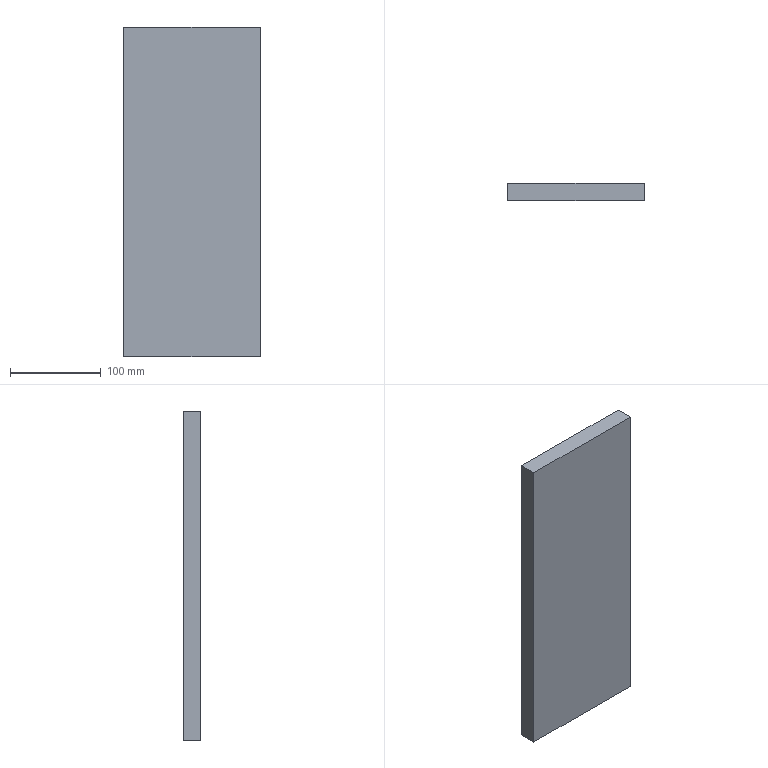Part | STEP file | SN10_010_005-02_PLACA | 1 solid | 6 faces | box 150 x 19 x 362.5 mm | volume 1033125 mm3 | plane 6
STEP:
#1=CARTESIAN_POINT('',(0.,0.,0.));
#2=DIRECTION('',(0.,0.,1.));
#3=DIRECTION('',(1.,0.,0.));
#4=AXIS2_PLACEMENT_3D('',#1,#2,#3);
#5=CARTESIAN_POINT('',(-75.,-419.,379.5));
#6=VERTEX_POINT('',#5);
#7=CARTESIAN_POINT('',(75.,-419.,379.5));
#8=VERTEX_POINT('',#7);
#9=CARTESIAN_POINT('',(-75.,-419.,379.5));
#10=DIRECTION('',(1.,0.,0.));
#11=VECTOR('',#10,1.);
#12=LINE('',#9,#11);
#13=CARTESIAN_POINT('',(0.,-419.,379.5));
#14=DIRECTION('',(0.,-1.,0.));
#15=DIRECTION('',(0.,0.,-1.));
#16=AXIS2_PLACEMENT_3D('',#13,#14,#15);
#17=PLANE('',#16);
#18=CARTESIAN_POINT('',(0.,-75.));
#19=DIRECTION('',(0.,1.));
#20=VECTOR('',#19,1.);
#21=LINE('',#18,#20);
#22=(GEOMETRIC_REPRESENTATION_CONTEXT(2)PARAMETRIC_REPRESENTATION_CONTEXT()REPRESENTATION_CONTEXT('',''));
#23=DEFINITIONAL_REPRESENTATION('',(#21),#22);
#24=PCURVE('',#17,#23);
#25=CARTESIAN_POINT('',(0.,-419.,379.5));
#26=DIRECTION('',(0.,0.,-1.));
#27=DIRECTION('',(-1.,0.,0.));
#28=AXIS2_PLACEMENT_3D('',#25,#26,#27);
#29=PLANE('',#28);
#30=CARTESIAN_POINT('',(75.,0.));
#31=DIRECTION('',(-1.,0.));
#32=VECTOR('',#31,1.);
#33=LINE('',#30,#32);
#34=(GEOMETRIC_REPRESENTATION_CONTEXT(2)PARAMETRIC_REPRESENTATION_CONTEXT()REPRESENTATION_CONTEXT('',''));
#35=DEFINITIONAL_REPRESENTATION('',(#33),#34);
#36=PCURVE('',#29,#35);
#37=SURFACE_CURVE('',#12,(#24,#36),.PCURVE_S1.);
#38=EDGE_CURVE('',#6,#8,#37,.T.);
#39=ORIENTED_EDGE('',*,*,#38,.F.);
#40=CARTESIAN_POINT('',(-75.,-419.,17.));
#41=VERTEX_POINT('',#40);
#42=CARTESIAN_POINT('',(-75.,-419.,379.5));
#43=DIRECTION('',(0.,0.,-1.));
#44=VECTOR('',#43,1.);
#45=LINE('',#42,#44);
#46=CARTESIAN_POINT('',(0.,-75.));
#47=DIRECTION('',(1.,0.));
#48=VECTOR('',#47,1.);
#49=LINE('',#46,#48);
#50=(GEOMETRIC_REPRESENTATION_CONTEXT(2)PARAMETRIC_REPRESENTATION_CONTEXT()REPRESENTATION_CONTEXT('',''));
#51=DEFINITIONAL_REPRESENTATION('',(#49),#50);
#52=PCURVE('',#17,#51);
#53=CARTESIAN_POINT('',(-75.,0.,0.));
#54=DIRECTION('',(1.,0.,0.));
#55=DIRECTION('',(0.,0.,-1.));
#56=AXIS2_PLACEMENT_3D('',#53,#54,#55);
#57=PLANE('',#56);
#58=CARTESIAN_POINT('',(-379.5,-419.));
#59=DIRECTION('',(1.,0.));
#60=VECTOR('',#59,1.);
#61=LINE('',#58,#60);
#62=(GEOMETRIC_REPRESENTATION_CONTEXT(2)PARAMETRIC_REPRESENTATION_CONTEXT()REPRESENTATION_CONTEXT('',''));
#63=DEFINITIONAL_REPRESENTATION('',(#61),#62);
#64=PCURVE('',#57,#63);
#65=SURFACE_CURVE('',#45,(#52,#64),.PCURVE_S1.);
#66=EDGE_CURVE('',#6,#41,#65,.T.);
#67=ORIENTED_EDGE('',*,*,#66,.T.);
#68=CARTESIAN_POINT('',(75.,-419.,17.));
#69=VERTEX_POINT('',#68);
#70=CARTESIAN_POINT('',(-75.,-419.,17.));
#71=DIRECTION('',(1.,0.,0.));
#72=VECTOR('',#71,1.);
#73=LINE('',#70,#72);
#74=CARTESIAN_POINT('',(362.5,-75.));
#75=DIRECTION('',(0.,1.));
#76=VECTOR('',#75,1.);
#77=LINE('',#74,#76);
#78=(GEOMETRIC_REPRESENTATION_CONTEXT(2)PARAMETRIC_REPRESENTATION_CONTEXT()REPRESENTATION_CONTEXT('',''));
#79=DEFINITIONAL_REPRESENTATION('',(#77),#78);
#80=PCURVE('',#17,#79);
#81=CARTESIAN_POINT('',(0.,-400.,17.));
#82=DIRECTION('',(0.,0.,1.));
#83=DIRECTION('',(1.,0.,0.));
#84=AXIS2_PLACEMENT_3D('',#81,#82,#83);
#85=PLANE('',#84);
#86=CARTESIAN_POINT('',(-75.,-19.));
#87=DIRECTION('',(1.,0.));
#88=VECTOR('',#87,1.);
#89=LINE('',#86,#88);
#90=(GEOMETRIC_REPRESENTATION_CONTEXT(2)PARAMETRIC_REPRESENTATION_CONTEXT()REPRESENTATION_CONTEXT('',''));
#91=DEFINITIONAL_REPRESENTATION('',(#89),#90);
#92=PCURVE('',#85,#91);
#93=SURFACE_CURVE('',#73,(#80,#92),.PCURVE_S1.);
#94=EDGE_CURVE('',#41,#69,#93,.T.);
#95=ORIENTED_EDGE('',*,*,#94,.T.);
#96=CARTESIAN_POINT('',(75.,-419.,379.5));
#97=DIRECTION('',(0.,0.,-1.));
#98=VECTOR('',#97,1.);
#99=LINE('',#96,#98);
#100=CARTESIAN_POINT('',(0.,75.));
#101=DIRECTION('',(1.,0.));
#102=VECTOR('',#101,1.);
#103=LINE('',#100,#102);
#104=(GEOMETRIC_REPRESENTATION_CONTEXT(2)PARAMETRIC_REPRESENTATION_CONTEXT()REPRESENTATION_CONTEXT('',''));
#105=DEFINITIONAL_REPRESENTATION('',(#103),#104);
#106=PCURVE('',#17,#105);
#107=CARTESIAN_POINT('',(75.,0.,0.));
#108=DIRECTION('',(1.,0.,0.));
#109=DIRECTION('',(0.,0.,-1.));
#110=AXIS2_PLACEMENT_3D('',#107,#108,#109);
#111=PLANE('',#110);
#112=CARTESIAN_POINT('',(-379.5,-419.));
#113=DIRECTION('',(1.,0.));
#114=VECTOR('',#113,1.);
#115=LINE('',#112,#114);
#116=(GEOMETRIC_REPRESENTATION_CONTEXT(2)PARAMETRIC_REPRESENTATION_CONTEXT()REPRESENTATION_CONTEXT('',''));
#117=DEFINITIONAL_REPRESENTATION('',(#115),#116);
#118=PCURVE('',#111,#117);
#119=SURFACE_CURVE('',#99,(#106,#118),.PCURVE_S1.);
#120=EDGE_CURVE('',#8,#69,#119,.T.);
#121=ORIENTED_EDGE('',*,*,#120,.F.);
#122=EDGE_LOOP('',(#39,#67,#95,#121));
#123=FACE_BOUND('',#122,.T.);
#124=ADVANCED_FACE('',(#123),#17,.T.);
#125=ORIENTED_EDGE('',*,*,#94,.F.);
#126=CARTESIAN_POINT('',(-75.,-400.,17.));
#127=VERTEX_POINT('',#126);
#128=CARTESIAN_POINT('',(-75.,-400.,17.));
#129=DIRECTION('',(0.,-1.,0.));
#130=VECTOR('',#129,1.);
#131=LINE('',#128,#130);
#132=CARTESIAN_POINT('',(-75.,0.));
#133=DIRECTION('',(0.,-1.));
#134=VECTOR('',#133,1.);
#135=LINE('',#132,#134);
#136=(GEOMETRIC_REPRESENTATION_CONTEXT(2)PARAMETRIC_REPRESENTATION_CONTEXT()REPRESENTATION_CONTEXT('',''));
#137=DEFINITIONAL_REPRESENTATION('',(#135),#136);
#138=PCURVE('',#85,#137);
#139=CARTESIAN_POINT('',(-17.,-400.));
#140=DIRECTION('',(0.,-1.));
#141=VECTOR('',#140,1.);
#142=LINE('',#139,#141);
#143=(GEOMETRIC_REPRESENTATION_CONTEXT(2)PARAMETRIC_REPRESENTATION_CONTEXT()REPRESENTATION_CONTEXT('',''));
#144=DEFINITIONAL_REPRESENTATION('',(#142),#143);
#145=PCURVE('',#57,#144);
#146=SURFACE_CURVE('',#131,(#138,#145),.PCURVE_S1.);
#147=EDGE_CURVE('',#127,#41,#146,.T.);
#148=ORIENTED_EDGE('',*,*,#147,.F.);
#149=CARTESIAN_POINT('',(75.,-400.,17.));
#150=VERTEX_POINT('',#149);
#151=CARTESIAN_POINT('',(-75.,-400.,17.));
#152=DIRECTION('',(1.,0.,0.));
#153=VECTOR('',#152,1.);
#154=LINE('',#151,#153);
#155=CARTESIAN_POINT('',(-75.,0.));
#156=DIRECTION('',(1.,0.));
#157=VECTOR('',#156,1.);
#158=LINE('',#155,#157);
#159=(GEOMETRIC_REPRESENTATION_CONTEXT(2)PARAMETRIC_REPRESENTATION_CONTEXT()REPRESENTATION_CONTEXT('',''));
#160=DEFINITIONAL_REPRESENTATION('',(#158),#159);
#161=PCURVE('',#85,#160);
#162=CARTESIAN_POINT('',(0.,-400.,17.));
#163=DIRECTION('',(0.,1.,0.));
#164=DIRECTION('',(0.,0.,1.));
#165=AXIS2_PLACEMENT_3D('',#162,#163,#164);
#166=PLANE('',#165);
#167=CARTESIAN_POINT('',(0.,-75.));
#168=DIRECTION('',(0.,1.));
#169=VECTOR('',#168,1.);
#170=LINE('',#167,#169);
#171=(GEOMETRIC_REPRESENTATION_CONTEXT(2)PARAMETRIC_REPRESENTATION_CONTEXT()REPRESENTATION_CONTEXT('',''));
#172=DEFINITIONAL_REPRESENTATION('',(#170),#171);
#173=PCURVE('',#166,#172);
#174=SURFACE_CURVE('',#154,(#161,#173),.PCURVE_S1.);
#175=EDGE_CURVE('',#127,#150,#174,.T.);
#176=ORIENTED_EDGE('',*,*,#175,.T.);
#177=CARTESIAN_POINT('',(75.,-400.,17.));
#178=DIRECTION('',(0.,-1.,0.));
#179=VECTOR('',#178,1.);
#180=LINE('',#177,#179);
#181=CARTESIAN_POINT('',(75.,0.));
#182=DIRECTION('',(0.,-1.));
#183=VECTOR('',#182,1.);
#184=LINE('',#181,#183);
#185=(GEOMETRIC_REPRESENTATION_CONTEXT(2)PARAMETRIC_REPRESENTATION_CONTEXT()REPRESENTATION_CONTEXT('',''));
#186=DEFINITIONAL_REPRESENTATION('',(#184),#185);
#187=PCURVE('',#85,#186);
#188=CARTESIAN_POINT('',(-17.,-400.));
#189=DIRECTION('',(0.,-1.));
#190=VECTOR('',#189,1.);
#191=LINE('',#188,#190);
#192=(GEOMETRIC_REPRESENTATION_CONTEXT(2)PARAMETRIC_REPRESENTATION_CONTEXT()REPRESENTATION_CONTEXT('',''));
#193=DEFINITIONAL_REPRESENTATION('',(#191),#192);
#194=PCURVE('',#111,#193);
#195=SURFACE_CURVE('',#180,(#187,#194),.PCURVE_S1.);
#196=EDGE_CURVE('',#150,#69,#195,.T.);
#197=ORIENTED_EDGE('',*,*,#196,.T.);
#198=EDGE_LOOP('',(#125,#148,#176,#197));
#199=FACE_BOUND('',#198,.T.);
#200=ADVANCED_FACE('',(#199),#85,.F.);
#201=ORIENTED_EDGE('',*,*,#175,.F.);
#202=CARTESIAN_POINT('',(-75.,-400.,379.5));
#203=VERTEX_POINT('',#202);
#204=CARTESIAN_POINT('',(-75.,-400.,17.));
#205=DIRECTION('',(0.,0.,1.));
#206=VECTOR('',#205,1.);
#207=LINE('',#204,#206);
#208=CARTESIAN_POINT('',(0.,-75.));
#209=DIRECTION('',(1.,0.));
#210=VECTOR('',#209,1.);
#211=LINE('',#208,#210);
#212=(GEOMETRIC_REPRESENTATION_CONTEXT(2)PARAMETRIC_REPRESENTATION_CONTEXT()REPRESENTATION_CONTEXT('',''));
#213=DEFINITIONAL_REPRESENTATION('',(#211),#212);
#214=PCURVE('',#166,#213);
#215=CARTESIAN_POINT('',(-17.,-400.));
#216=DIRECTION('',(-1.,0.));
#217=VECTOR('',#216,1.);
#218=LINE('',#215,#217);
#219=(GEOMETRIC_REPRESENTATION_CONTEXT(2)PARAMETRIC_REPRESENTATION_CONTEXT()REPRESENTATION_CONTEXT('',''));
#220=DEFINITIONAL_REPRESENTATION('',(#218),#219);
#221=PCURVE('',#57,#220);
#222=SURFACE_CURVE('',#207,(#214,#221),.PCURVE_S1.);
#223=EDGE_CURVE('',#127,#203,#222,.T.);
#224=ORIENTED_EDGE('',*,*,#223,.T.);
#225=CARTESIAN_POINT('',(75.,-400.,379.5));
#226=VERTEX_POINT('',#225);
#227=CARTESIAN_POINT('',(-75.,-400.,379.5));
#228=DIRECTION('',(1.,0.,0.));
#229=VECTOR('',#228,1.);
#230=LINE('',#227,#229);
#231=CARTESIAN_POINT('',(362.5,-75.));
#232=DIRECTION('',(0.,1.));
#233=VECTOR('',#232,1.);
#234=LINE('',#231,#233);
#235=(GEOMETRIC_REPRESENTATION_CONTEXT(2)PARAMETRIC_REPRESENTATION_CONTEXT()REPRESENTATION_CONTEXT('',''));
#236=DEFINITIONAL_REPRESENTATION('',(#234),#235);
#237=PCURVE('',#166,#236);
#238=CARTESIAN_POINT('',(75.,19.));
#239=DIRECTION('',(-1.,0.));
#240=VECTOR('',#239,1.);
#241=LINE('',#238,#240);
#242=(GEOMETRIC_REPRESENTATION_CONTEXT(2)PARAMETRIC_REPRESENTATION_CONTEXT()REPRESENTATION_CONTEXT('',''));
#243=DEFINITIONAL_REPRESENTATION('',(#241),#242);
#244=PCURVE('',#29,#243);
#245=SURFACE_CURVE('',#230,(#237,#244),.PCURVE_S1.);
#246=EDGE_CURVE('',#203,#226,#245,.T.);
#247=ORIENTED_EDGE('',*,*,#246,.T.);
#248=CARTESIAN_POINT('',(75.,-400.,17.));
#249=DIRECTION('',(0.,0.,1.));
#250=VECTOR('',#249,1.);
#251=LINE('',#248,#250);
#252=CARTESIAN_POINT('',(0.,75.));
#253=DIRECTION('',(1.,0.));
#254=VECTOR('',#253,1.);
#255=LINE('',#252,#254);
#256=(GEOMETRIC_REPRESENTATION_CONTEXT(2)PARAMETRIC_REPRESENTATION_CONTEXT()REPRESENTATION_CONTEXT('',''));
#257=DEFINITIONAL_REPRESENTATION('',(#255),#256);
#258=PCURVE('',#166,#257);
#259=CARTESIAN_POINT('',(-17.,-400.));
#260=DIRECTION('',(-1.,0.));
#261=VECTOR('',#260,1.);
#262=LINE('',#259,#261);
#263=(GEOMETRIC_REPRESENTATION_CONTEXT(2)PARAMETRIC_REPRESENTATION_CONTEXT()REPRESENTATION_CONTEXT('',''));
#264=DEFINITIONAL_REPRESENTATION('',(#262),#263);
#265=PCURVE('',#111,#264);
#266=SURFACE_CURVE('',#251,(#258,#265),.PCURVE_S1.);
#267=EDGE_CURVE('',#150,#226,#266,.T.);
#268=ORIENTED_EDGE('',*,*,#267,.F.);
#269=EDGE_LOOP('',(#201,#224,#247,#268));
#270=FACE_BOUND('',#269,.T.);
#271=ADVANCED_FACE('',(#270),#166,.T.);
#272=ORIENTED_EDGE('',*,*,#246,.F.);
#273=CARTESIAN_POINT('',(-75.,-419.,379.5));
#274=DIRECTION('',(0.,1.,0.));
#275=VECTOR('',#274,1.);
#276=LINE('',#273,#275);
#277=CARTESIAN_POINT('',(75.,0.));
#278=DIRECTION('',(0.,1.));
#279=VECTOR('',#278,1.);
#280=LINE('',#277,#279);
#281=(GEOMETRIC_REPRESENTATION_CONTEXT(2)PARAMETRIC_REPRESENTATION_CONTEXT()REPRESENTATION_CONTEXT('',''));
#282=DEFINITIONAL_REPRESENTATION('',(#280),#281);
#283=PCURVE('',#29,#282);
#284=CARTESIAN_POINT('',(-379.5,-419.));
#285=DIRECTION('',(0.,1.));
#286=VECTOR('',#285,1.);
#287=LINE('',#284,#286);
#288=(GEOMETRIC_REPRESENTATION_CONTEXT(2)PARAMETRIC_REPRESENTATION_CONTEXT()REPRESENTATION_CONTEXT('',''));
#289=DEFINITIONAL_REPRESENTATION('',(#287),#288);
#290=PCURVE('',#57,#289);
#291=SURFACE_CURVE('',#276,(#283,#290),.PCURVE_S1.);
#292=EDGE_CURVE('',#6,#203,#291,.T.);
#293=ORIENTED_EDGE('',*,*,#292,.F.);
#294=ORIENTED_EDGE('',*,*,#38,.T.);
#295=CARTESIAN_POINT('',(75.,-419.,379.5));
#296=DIRECTION('',(0.,1.,0.));
#297=VECTOR('',#296,1.);
#298=LINE('',#295,#297);
#299=CARTESIAN_POINT('',(-75.,0.));
#300=DIRECTION('',(0.,1.));
#301=VECTOR('',#300,1.);
#302=LINE('',#299,#301);
#303=(GEOMETRIC_REPRESENTATION_CONTEXT(2)PARAMETRIC_REPRESENTATION_CONTEXT()REPRESENTATION_CONTEXT('',''));
#304=DEFINITIONAL_REPRESENTATION('',(#302),#303);
#305=PCURVE('',#29,#304);
#306=CARTESIAN_POINT('',(-379.5,-419.));
#307=DIRECTION('',(0.,1.));
#308=VECTOR('',#307,1.);
#309=LINE('',#306,#308);
#310=(GEOMETRIC_REPRESENTATION_CONTEXT(2)PARAMETRIC_REPRESENTATION_CONTEXT()REPRESENTATION_CONTEXT('',''));
#311=DEFINITIONAL_REPRESENTATION('',(#309),#310);
#312=PCURVE('',#111,#311);
#313=SURFACE_CURVE('',#298,(#305,#312),.PCURVE_S1.);
#314=EDGE_CURVE('',#8,#226,#313,.T.);
#315=ORIENTED_EDGE('',*,*,#314,.T.);
#316=EDGE_LOOP('',(#272,#293,#294,#315));
#317=FACE_BOUND('',#316,.T.);
#318=ADVANCED_FACE('',(#317),#29,.F.);
#319=ORIENTED_EDGE('',*,*,#292,.T.);
#320=ORIENTED_EDGE('',*,*,#223,.F.);
#321=ORIENTED_EDGE('',*,*,#147,.T.);
#322=ORIENTED_EDGE('',*,*,#66,.F.);
#323=EDGE_LOOP('',(#319,#320,#321,#322));
#324=FACE_BOUND('',#323,.T.);
#325=ADVANCED_FACE('',(#324),#57,.F.);
#326=ORIENTED_EDGE('',*,*,#120,.T.);
#327=ORIENTED_EDGE('',*,*,#196,.F.);
#328=ORIENTED_EDGE('',*,*,#267,.T.);
#329=ORIENTED_EDGE('',*,*,#314,.F.);
#330=EDGE_LOOP('',(#326,#327,#328,#329));
#331=FACE_BOUND('',#330,.T.);
#332=ADVANCED_FACE('',(#331),#111,.T.);
#333=CLOSED_SHELL('',(#124,#200,#271,#318,#325,#332));
#334=MANIFOLD_SOLID_BREP('',#333);
#335=(LENGTH_UNIT()NAMED_UNIT(*)SI_UNIT(.MILLI.,.METRE.));
#336=UNCERTAINTY_MEASURE_WITH_UNIT(LENGTH_MEASURE(0.0000001),#335,'','');
#337=(NAMED_UNIT(*)PLANE_ANGLE_UNIT()SI_UNIT($,.RADIAN.));
#338=(NAMED_UNIT(*)SI_UNIT($,.STERADIAN.)SOLID_ANGLE_UNIT());
#339=(GEOMETRIC_REPRESENTATION_CONTEXT(3)GLOBAL_UNCERTAINTY_ASSIGNED_CONTEXT((#336))GLOBAL_UNIT_ASSIGNED_CONTEXT((#335,#337,#338))REPRESENTATION_CONTEXT('',''));
#340=ADVANCED_BREP_SHAPE_REPRESENTATION('',(#4,#334),#339);